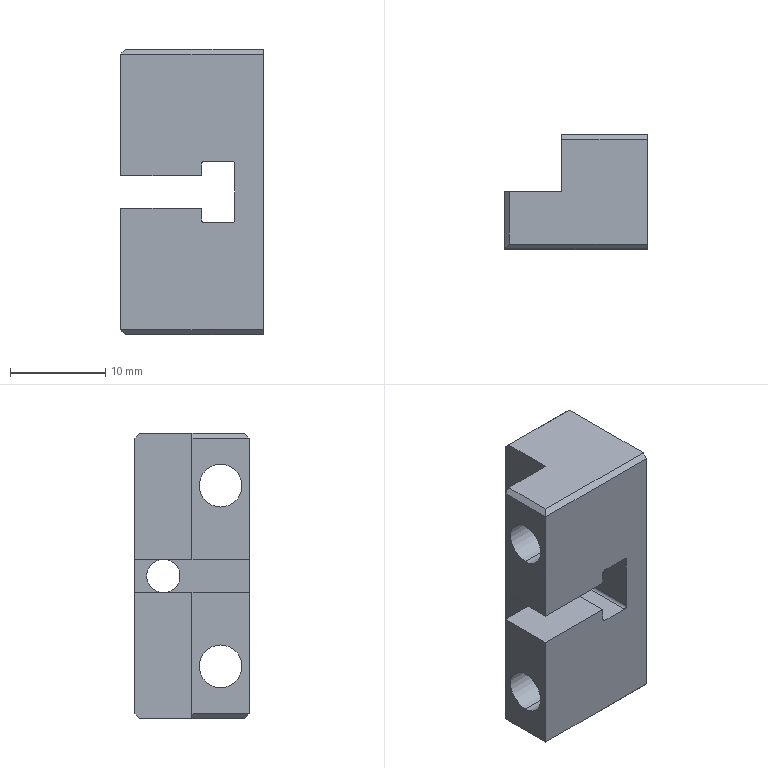Part | NX | features BREP 1 | 1 solid | 34 faces | box 15 x 12 x 30 mm | volume 3310 mm3 | plane 24 | cylinder 10 | commonest cylinder face diameters 0.6 x4 4.5 x4 3.5 x2
STEP:
#1=CARTESIAN_POINT('',(-3.,9.,16.75));
#2=VERTEX_POINT('',#1);
#3=CARTESIAN_POINT('',(-3.,9.,13.25));
#4=VERTEX_POINT('',#3);
#5=CARTESIAN_POINT('',(-3.,9.,15.));
#6=DIRECTION('',(1.,0.,0.));
#7=DIRECTION('',(0.,1.,0.));
#8=AXIS2_PLACEMENT_3D('',#5,#6,#7);
#9=CIRCLE('',#8,1.75);
#10=EDGE_CURVE('',#2,#4,#9,.T.);
#11=ORIENTED_EDGE('',*,*,#10,.F.);
#12=CARTESIAN_POINT('',(0.,9.,16.75));
#13=VERTEX_POINT('',#12);
#14=CARTESIAN_POINT('',(0.,9.,16.75));
#15=DIRECTION('',(1.,0.,0.));
#16=VECTOR('',#15,1000.);
#17=LINE('',#14,#16);
#18=EDGE_CURVE('',#2,#13,#17,.T.);
#19=ORIENTED_EDGE('',*,*,#18,.T.);
#20=CARTESIAN_POINT('',(0.,9.,13.25));
#21=VERTEX_POINT('',#20);
#22=CARTESIAN_POINT('',(0.,9.,15.));
#23=DIRECTION('',(1.,0.,0.));
#24=DIRECTION('',(0.,0.,-1.));
#25=AXIS2_PLACEMENT_3D('',#22,#23,#24);
#26=CIRCLE('',#25,1.75);
#27=EDGE_CURVE('',#13,#21,#26,.T.);
#28=ORIENTED_EDGE('',*,*,#27,.T.);
#29=CARTESIAN_POINT('',(0.,9.,13.25));
#30=DIRECTION('',(1.,0.,0.));
#31=VECTOR('',#30,1000.);
#32=LINE('',#29,#31);
#33=EDGE_CURVE('',#4,#21,#32,.T.);
#34=ORIENTED_EDGE('',*,*,#33,.F.);
#35=EDGE_LOOP('',(#11,#19,#28,#34));
#36=FACE_BOUND('',#35,.T.);
#37=CARTESIAN_POINT('',(0.,9.,15.));
#38=DIRECTION('',(1.,0.,0.));
#39=DIRECTION('',(0.,0.,-1.));
#40=AXIS2_PLACEMENT_3D('',#37,#38,#39);
#41=CYLINDRICAL_SURFACE('',#40,1.75);
#42=ADVANCED_FACE('',(#36),#41,.F.);
#43=CARTESIAN_POINT('',(-15.,3.,26.75));
#44=VERTEX_POINT('',#43);
#45=CARTESIAN_POINT('',(-15.,3.,22.25));
#46=VERTEX_POINT('',#45);
#47=CARTESIAN_POINT('',(-15.,3.,24.5));
#48=DIRECTION('',(1.,0.,0.));
#49=DIRECTION('',(0.,0.,-1.));
#50=AXIS2_PLACEMENT_3D('',#47,#48,#49);
#51=CIRCLE('',#50,2.25);
#52=EDGE_CURVE('',#44,#46,#51,.T.);
#53=ORIENTED_EDGE('',*,*,#52,.F.);
#54=CARTESIAN_POINT('',(0.,3.,26.75));
#55=VERTEX_POINT('',#54);
#56=CARTESIAN_POINT('',(0.,3.,26.75));
#57=DIRECTION('',(1.,0.,0.));
#58=VECTOR('',#57,1000.);
#59=LINE('',#56,#58);
#60=EDGE_CURVE('',#44,#55,#59,.T.);
#61=ORIENTED_EDGE('',*,*,#60,.T.);
#62=CARTESIAN_POINT('',(0.,3.,22.25));
#63=VERTEX_POINT('',#62);
#64=CARTESIAN_POINT('',(0.,3.,24.5));
#65=DIRECTION('',(1.,0.,0.));
#66=DIRECTION('',(0.,0.,-1.));
#67=AXIS2_PLACEMENT_3D('',#64,#65,#66);
#68=CIRCLE('',#67,2.25);
#69=EDGE_CURVE('',#55,#63,#68,.T.);
#70=ORIENTED_EDGE('',*,*,#69,.T.);
#71=CARTESIAN_POINT('',(0.,3.,22.25));
#72=DIRECTION('',(1.,0.,0.));
#73=VECTOR('',#72,1000.);
#74=LINE('',#71,#73);
#75=EDGE_CURVE('',#46,#63,#74,.T.);
#76=ORIENTED_EDGE('',*,*,#75,.F.);
#77=EDGE_LOOP('',(#53,#61,#70,#76));
#78=FACE_BOUND('',#77,.T.);
#79=CARTESIAN_POINT('',(0.,3.,24.5));
#80=DIRECTION('',(1.,0.,0.));
#81=DIRECTION('',(0.,0.,-1.));
#82=AXIS2_PLACEMENT_3D('',#79,#80,#81);
#83=CYLINDRICAL_SURFACE('',#82,2.25);
#84=ADVANCED_FACE('',(#78),#83,.F.);
#85=CARTESIAN_POINT('',(-15.,3.,7.75));
#86=VERTEX_POINT('',#85);
#87=CARTESIAN_POINT('',(-15.,3.,3.25));
#88=VERTEX_POINT('',#87);
#89=CARTESIAN_POINT('',(-15.,3.,5.5));
#90=DIRECTION('',(1.,0.,0.));
#91=DIRECTION('',(0.,0.,-1.));
#92=AXIS2_PLACEMENT_3D('',#89,#90,#91);
#93=CIRCLE('',#92,2.25);
#94=EDGE_CURVE('',#86,#88,#93,.T.);
#95=ORIENTED_EDGE('',*,*,#94,.F.);
#96=CARTESIAN_POINT('',(0.,3.,7.75));
#97=VERTEX_POINT('',#96);
#98=CARTESIAN_POINT('',(0.,3.,7.75));
#99=DIRECTION('',(1.,0.,0.));
#100=VECTOR('',#99,1000.);
#101=LINE('',#98,#100);
#102=EDGE_CURVE('',#86,#97,#101,.T.);
#103=ORIENTED_EDGE('',*,*,#102,.T.);
#104=CARTESIAN_POINT('',(0.,3.,3.25));
#105=VERTEX_POINT('',#104);
#106=CARTESIAN_POINT('',(0.,3.,5.5));
#107=DIRECTION('',(1.,0.,0.));
#108=DIRECTION('',(0.,0.,-1.));
#109=AXIS2_PLACEMENT_3D('',#106,#107,#108);
#110=CIRCLE('',#109,2.25);
#111=EDGE_CURVE('',#97,#105,#110,.T.);
#112=ORIENTED_EDGE('',*,*,#111,.T.);
#113=CARTESIAN_POINT('',(0.,3.,3.25));
#114=DIRECTION('',(1.,0.,0.));
#115=VECTOR('',#114,1000.);
#116=LINE('',#113,#115);
#117=EDGE_CURVE('',#88,#105,#116,.T.);
#118=ORIENTED_EDGE('',*,*,#117,.F.);
#119=EDGE_LOOP('',(#95,#103,#112,#118));
#120=FACE_BOUND('',#119,.T.);
#121=CARTESIAN_POINT('',(0.,3.,5.5));
#122=DIRECTION('',(1.,0.,0.));
#123=DIRECTION('',(0.,0.,-1.));
#124=AXIS2_PLACEMENT_3D('',#121,#122,#123);
#125=CYLINDRICAL_SURFACE('',#124,2.25);
#126=ADVANCED_FACE('',(#120),#125,.F.);
#127=CARTESIAN_POINT('',(-9.,6.,30.));
#128=VERTEX_POINT('',#127);
#129=CARTESIAN_POINT('',(-9.,6.,16.7));
#130=VERTEX_POINT('',#129);
#131=CARTESIAN_POINT('',(-9.,6.,30.));
#132=DIRECTION('',(0.,0.,-1.));
#133=VECTOR('',#132,1000.);
#134=LINE('',#131,#133);
#135=EDGE_CURVE('',#128,#130,#134,.T.);
#136=ORIENTED_EDGE('',*,*,#135,.T.);
#137=CARTESIAN_POINT('',(-15.,6.,16.7));
#138=VERTEX_POINT('',#137);
#139=CARTESIAN_POINT('',(-9.,6.,16.7));
#140=DIRECTION('',(1.,0.,0.));
#141=VECTOR('',#140,1000.);
#142=LINE('',#139,#141);
#143=EDGE_CURVE('',#138,#130,#142,.T.);
#144=ORIENTED_EDGE('',*,*,#143,.F.);
#145=CARTESIAN_POINT('',(-15.,6.,29.5));
#146=VERTEX_POINT('',#145);
#147=CARTESIAN_POINT('',(-15.,6.,30.));
#148=DIRECTION('',(0.,0.,-1.));
#149=VECTOR('',#148,1000.);
#150=LINE('',#147,#149);
#151=EDGE_CURVE('',#146,#138,#150,.T.);
#152=ORIENTED_EDGE('',*,*,#151,.F.);
#153=CARTESIAN_POINT('',(-14.5,6.,30.));
#154=VERTEX_POINT('',#153);
#155=CARTESIAN_POINT('',(-14.5,6.,30.));
#156=DIRECTION('',(0.7071,0.,0.7071));
#157=VECTOR('',#156,1000.);
#158=LINE('',#155,#157);
#159=EDGE_CURVE('',#146,#154,#158,.T.);
#160=ORIENTED_EDGE('',*,*,#159,.T.);
#161=CARTESIAN_POINT('',(-9.,6.,30.));
#162=DIRECTION('',(-1.,0.,0.));
#163=VECTOR('',#162,1000.);
#164=LINE('',#161,#163);
#165=EDGE_CURVE('',#128,#154,#164,.T.);
#166=ORIENTED_EDGE('',*,*,#165,.F.);
#167=EDGE_LOOP('',(#136,#144,#152,#160,#166));
#168=FACE_BOUND('',#167,.T.);
#169=CARTESIAN_POINT('',(-9.,6.,30.));
#170=DIRECTION('',(0.,-1.,0.));
#171=DIRECTION('',(0.,0.,-1.));
#172=AXIS2_PLACEMENT_3D('',#169,#170,#171);
#173=PLANE('',#172);
#174=ADVANCED_FACE('',(#168),#173,.F.);
#175=ORIENTED_EDGE('',*,*,#151,.T.);
#176=CARTESIAN_POINT('',(-15.,0.,16.7));
#177=VERTEX_POINT('',#176);
#178=CARTESIAN_POINT('',(-15.,0.,16.7));
#179=DIRECTION('',(0.,1.,0.));
#180=VECTOR('',#179,1000.);
#181=LINE('',#178,#180);
#182=EDGE_CURVE('',#177,#138,#181,.T.);
#183=ORIENTED_EDGE('',*,*,#182,.F.);
#184=CARTESIAN_POINT('',(-15.,0.,29.5));
#185=VERTEX_POINT('',#184);
#186=CARTESIAN_POINT('',(-15.,0.,30.));
#187=DIRECTION('',(0.,0.,-1.));
#188=VECTOR('',#187,1000.);
#189=LINE('',#186,#188);
#190=EDGE_CURVE('',#185,#177,#189,.T.);
#191=ORIENTED_EDGE('',*,*,#190,.F.);
#192=CARTESIAN_POINT('',(-15.,6.,29.5));
#193=DIRECTION('',(0.,1.,0.));
#194=VECTOR('',#193,1000.);
#195=LINE('',#192,#194);
#196=EDGE_CURVE('',#185,#146,#195,.T.);
#197=ORIENTED_EDGE('',*,*,#196,.T.);
#198=EDGE_LOOP('',(#175,#183,#191,#197));
#199=FACE_BOUND('',#198,.T.);
#200=CARTESIAN_POINT('',(-15.,3.,24.5));
#201=DIRECTION('',(1.,0.,0.));
#202=DIRECTION('',(0.,0.,-1.));
#203=AXIS2_PLACEMENT_3D('',#200,#201,#202);
#204=CIRCLE('',#203,2.25);
#205=EDGE_CURVE('',#46,#44,#204,.T.);
#206=ORIENTED_EDGE('',*,*,#205,.T.);
#207=ORIENTED_EDGE('',*,*,#52,.T.);
#208=EDGE_LOOP('',(#206,#207));
#209=FACE_BOUND('',#208,.T.);
#210=CARTESIAN_POINT('',(-15.,6.,30.));
#211=DIRECTION('',(1.,0.,0.));
#212=DIRECTION('',(0.,1.,0.));
#213=AXIS2_PLACEMENT_3D('',#210,#211,#212);
#214=PLANE('',#213);
#215=ADVANCED_FACE('',(#199,#209),#214,.F.);
#216=CARTESIAN_POINT('',(0.,0.,29.5));
#217=VERTEX_POINT('',#216);
#218=CARTESIAN_POINT('',(0.,0.,0.5));
#219=VERTEX_POINT('',#218);
#220=CARTESIAN_POINT('',(0.,0.,30.));
#221=DIRECTION('',(0.,0.,-1.));
#222=VECTOR('',#221,1000.);
#223=LINE('',#220,#222);
#224=EDGE_CURVE('',#217,#219,#223,.T.);
#225=ORIENTED_EDGE('',*,*,#224,.T.);
#226=CARTESIAN_POINT('',(0.,0.5,0.));
#227=VERTEX_POINT('',#226);
#228=CARTESIAN_POINT('',(0.,0.,0.5));
#229=DIRECTION('',(0.,0.7071,-0.7071));
#230=VECTOR('',#229,1000.);
#231=LINE('',#228,#230);
#232=EDGE_CURVE('',#219,#227,#231,.T.);
#233=ORIENTED_EDGE('',*,*,#232,.T.);
#234=CARTESIAN_POINT('',(0.,11.5,0.));
#235=VERTEX_POINT('',#234);
#236=CARTESIAN_POINT('',(0.,0.,0.));
#237=DIRECTION('',(0.,1.,0.));
#238=VECTOR('',#237,1000.);
#239=LINE('',#236,#238);
#240=EDGE_CURVE('',#227,#235,#239,.T.);
#241=ORIENTED_EDGE('',*,*,#240,.T.);
#242=CARTESIAN_POINT('',(0.,12.,0.5));
#243=VERTEX_POINT('',#242);
#244=CARTESIAN_POINT('',(0.,12.,0.5));
#245=DIRECTION('',(0.,0.7071,0.7071));
#246=VECTOR('',#245,1000.);
#247=LINE('',#244,#246);
#248=EDGE_CURVE('',#235,#243,#247,.T.);
#249=ORIENTED_EDGE('',*,*,#248,.T.);
#250=CARTESIAN_POINT('',(0.,12.,29.5));
#251=VERTEX_POINT('',#250);
#252=CARTESIAN_POINT('',(0.,12.,30.));
#253=DIRECTION('',(0.,0.,-1.));
#254=VECTOR('',#253,1000.);
#255=LINE('',#252,#254);
#256=EDGE_CURVE('',#251,#243,#255,.T.);
#257=ORIENTED_EDGE('',*,*,#256,.F.);
#258=CARTESIAN_POINT('',(0.,11.5,30.));
#259=VERTEX_POINT('',#258);
#260=CARTESIAN_POINT('',(0.,11.5,30.));
#261=DIRECTION('',(0.,-0.7071,0.7071));
#262=VECTOR('',#261,1000.);
#263=LINE('',#260,#262);
#264=EDGE_CURVE('',#251,#259,#263,.T.);
#265=ORIENTED_EDGE('',*,*,#264,.T.);
#266=CARTESIAN_POINT('',(0.,0.5,30.));
#267=VERTEX_POINT('',#266);
#268=CARTESIAN_POINT('',(0.,0.,30.));
#269=DIRECTION('',(0.,1.,0.));
#270=VECTOR('',#269,1000.);
#271=LINE('',#268,#270);
#272=EDGE_CURVE('',#267,#259,#271,.T.);
#273=ORIENTED_EDGE('',*,*,#272,.F.);
#274=CARTESIAN_POINT('',(0.,0.5,30.));
#275=DIRECTION('',(0.,-0.7071,-0.7071));
#276=VECTOR('',#275,1000.);
#277=LINE('',#274,#276);
#278=EDGE_CURVE('',#267,#217,#277,.T.);
#279=ORIENTED_EDGE('',*,*,#278,.T.);
#280=EDGE_LOOP('',(#225,#233,#241,#249,#257,#265,#273,#279));
#281=FACE_BOUND('',#280,.T.);
#282=CARTESIAN_POINT('',(0.,3.,5.5));
#283=DIRECTION('',(1.,0.,0.));
#284=DIRECTION('',(0.,0.,-1.));
#285=AXIS2_PLACEMENT_3D('',#282,#283,#284);
#286=CIRCLE('',#285,2.25);
#287=EDGE_CURVE('',#105,#97,#286,.T.);
#288=ORIENTED_EDGE('',*,*,#287,.F.);
#289=ORIENTED_EDGE('',*,*,#111,.F.);
#290=EDGE_LOOP('',(#288,#289));
#291=FACE_BOUND('',#290,.T.);
#292=CARTESIAN_POINT('',(0.,3.,24.5));
#293=DIRECTION('',(1.,0.,0.));
#294=DIRECTION('',(0.,0.,-1.));
#295=AXIS2_PLACEMENT_3D('',#292,#293,#294);
#296=CIRCLE('',#295,2.25);
#297=EDGE_CURVE('',#63,#55,#296,.T.);
#298=ORIENTED_EDGE('',*,*,#297,.F.);
#299=ORIENTED_EDGE('',*,*,#69,.F.);
#300=EDGE_LOOP('',(#298,#299));
#301=FACE_BOUND('',#300,.T.);
#302=CARTESIAN_POINT('',(0.,9.,15.));
#303=DIRECTION('',(1.,0.,0.));
#304=DIRECTION('',(0.,0.,-1.));
#305=AXIS2_PLACEMENT_3D('',#302,#303,#304);
#306=CIRCLE('',#305,1.75);
#307=EDGE_CURVE('',#21,#13,#306,.T.);
#308=ORIENTED_EDGE('',*,*,#307,.F.);
#309=ORIENTED_EDGE('',*,*,#27,.F.);
#310=EDGE_LOOP('',(#308,#309));
#311=FACE_BOUND('',#310,.T.);
#312=CARTESIAN_POINT('',(0.,0.,30.));
#313=DIRECTION('',(-1.,0.,0.));
#314=DIRECTION('',(0.,0.,1.));
#315=AXIS2_PLACEMENT_3D('',#312,#313,#314);
#316=PLANE('',#315);
#317=ADVANCED_FACE('',(#281,#291,#301,#311),#316,.F.);
#318=CARTESIAN_POINT('',(-9.,6.,13.3));
#319=VERTEX_POINT('',#318);
#320=CARTESIAN_POINT('',(-9.,6.,0.));
#321=VERTEX_POINT('',#320);
#322=CARTESIAN_POINT('',(-9.,6.,30.));
#323=DIRECTION('',(0.,0.,-1.));
#324=VECTOR('',#323,1000.);
#325=LINE('',#322,#324);
#326=EDGE_CURVE('',#319,#321,#325,.T.);
#327=ORIENTED_EDGE('',*,*,#326,.F.);
#328=CARTESIAN_POINT('',(-9.,12.,13.3));
#329=VERTEX_POINT('',#328);
#330=CARTESIAN_POINT('',(-9.,0.,13.3));
#331=DIRECTION('',(0.,1.,0.));
#332=VECTOR('',#331,1000.);
#333=LINE('',#330,#332);
#334=EDGE_CURVE('',#319,#329,#333,.T.);
#335=ORIENTED_EDGE('',*,*,#334,.T.);
#336=CARTESIAN_POINT('',(-9.,12.,0.5));
#337=VERTEX_POINT('',#336);
#338=CARTESIAN_POINT('',(-9.,12.,30.));
#339=DIRECTION('',(0.,0.,-1.));
#340=VECTOR('',#339,1000.);
#341=LINE('',#338,#340);
#342=EDGE_CURVE('',#329,#337,#341,.T.);
#343=ORIENTED_EDGE('',*,*,#342,.T.);
#344=CARTESIAN_POINT('',(-9.,11.5,0.));
#345=VERTEX_POINT('',#344);
#346=CARTESIAN_POINT('',(-9.,12.,0.5));
#347=DIRECTION('',(0.,-0.7071,-0.7071));
#348=VECTOR('',#347,1000.);
#349=LINE('',#346,#348);
#350=EDGE_CURVE('',#337,#345,#349,.T.);
#351=ORIENTED_EDGE('',*,*,#350,.T.);
#352=CARTESIAN_POINT('',(-9.,12.,0.));
#353=DIRECTION('',(0.,-1.,0.));
#354=VECTOR('',#353,1000.);
#355=LINE('',#352,#354);
#356=EDGE_CURVE('',#345,#321,#355,.T.);
#357=ORIENTED_EDGE('',*,*,#356,.T.);
#358=EDGE_LOOP('',(#327,#335,#343,#351,#357));
#359=FACE_BOUND('',#358,.T.);
#360=CARTESIAN_POINT('',(-9.,12.,30.));
#361=DIRECTION('',(1.,0.,0.));
#362=DIRECTION('',(0.,1.,0.));
#363=AXIS2_PLACEMENT_3D('',#360,#361,#362);
#364=PLANE('',#363);
#365=ADVANCED_FACE('',(#359),#364,.F.);
#366=ORIENTED_EDGE('',*,*,#342,.F.);
#367=CARTESIAN_POINT('',(-6.5,12.,13.3));
#368=VERTEX_POINT('',#367);
#369=CARTESIAN_POINT('',(-9.,12.,13.3));
#370=DIRECTION('',(-1.,0.,0.));
#371=VECTOR('',#370,1000.);
#372=LINE('',#369,#371);
#373=EDGE_CURVE('',#368,#329,#372,.T.);
#374=ORIENTED_EDGE('',*,*,#373,.F.);
#375=CARTESIAN_POINT('',(-6.5,12.,12.05));
#376=VERTEX_POINT('',#375);
#377=CARTESIAN_POINT('',(-6.5,12.,13.3));
#378=DIRECTION('',(0.,0.,1.));
#379=VECTOR('',#378,1000.);
#380=LINE('',#377,#379);
#381=EDGE_CURVE('',#376,#368,#380,.T.);
#382=ORIENTED_EDGE('',*,*,#381,.F.);
#383=CARTESIAN_POINT('',(-6.2,12.,11.75));
#384=VERTEX_POINT('',#383);
#385=CARTESIAN_POINT('',(-6.2,12.,12.05));
#386=DIRECTION('',(0.,-1.,0.));
#387=DIRECTION('',(1.,0.,0.));
#388=AXIS2_PLACEMENT_3D('',#385,#386,#387);
#389=CIRCLE('',#388,0.3);
#390=EDGE_CURVE('',#376,#384,#389,.T.);
#391=ORIENTED_EDGE('',*,*,#390,.T.);
#392=CARTESIAN_POINT('',(-3.3,12.,11.75));
#393=VERTEX_POINT('',#392);
#394=CARTESIAN_POINT('',(-6.5,12.,11.75));
#395=DIRECTION('',(-1.,0.,0.));
#396=VECTOR('',#395,1000.);
#397=LINE('',#394,#396);
#398=EDGE_CURVE('',#393,#384,#397,.T.);
#399=ORIENTED_EDGE('',*,*,#398,.F.);
#400=CARTESIAN_POINT('',(-3.,12.,12.05));
#401=VERTEX_POINT('',#400);
#402=CARTESIAN_POINT('',(-3.3,12.,12.05));
#403=DIRECTION('',(0.,-1.,0.));
#404=DIRECTION('',(1.,0.,0.));
#405=AXIS2_PLACEMENT_3D('',#402,#403,#404);
#406=CIRCLE('',#405,0.3);
#407=EDGE_CURVE('',#393,#401,#406,.T.);
#408=ORIENTED_EDGE('',*,*,#407,.T.);
#409=CARTESIAN_POINT('',(-3.,12.,17.95));
#410=VERTEX_POINT('',#409);
#411=CARTESIAN_POINT('',(-3.,12.,11.75));
#412=DIRECTION('',(0.,0.,-1.));
#413=VECTOR('',#412,1000.);
#414=LINE('',#411,#413);
#415=EDGE_CURVE('',#410,#401,#414,.T.);
#416=ORIENTED_EDGE('',*,*,#415,.F.);
#417=CARTESIAN_POINT('',(-3.3,12.,18.25));
#418=VERTEX_POINT('',#417);
#419=CARTESIAN_POINT('',(-3.3,12.,17.95));
#420=DIRECTION('',(0.,-1.,0.));
#421=DIRECTION('',(1.,0.,0.));
#422=AXIS2_PLACEMENT_3D('',#419,#420,#421);
#423=CIRCLE('',#422,0.3);
#424=EDGE_CURVE('',#410,#418,#423,.T.);
#425=ORIENTED_EDGE('',*,*,#424,.T.);
#426=CARTESIAN_POINT('',(-6.2,12.,18.25));
#427=VERTEX_POINT('',#426);
#428=CARTESIAN_POINT('',(-3.,12.,18.25));
#429=DIRECTION('',(1.,0.,0.));
#430=VECTOR('',#429,1000.);
#431=LINE('',#428,#430);
#432=EDGE_CURVE('',#427,#418,#431,.T.);
#433=ORIENTED_EDGE('',*,*,#432,.F.);
#434=CARTESIAN_POINT('',(-6.5,12.,17.95));
#435=VERTEX_POINT('',#434);
#436=CARTESIAN_POINT('',(-6.2,12.,17.95));
#437=DIRECTION('',(0.,-1.,0.));
#438=DIRECTION('',(1.,0.,0.));
#439=AXIS2_PLACEMENT_3D('',#436,#437,#438);
#440=CIRCLE('',#439,0.3);
#441=EDGE_CURVE('',#427,#435,#440,.T.);
#442=ORIENTED_EDGE('',*,*,#441,.T.);
#443=CARTESIAN_POINT('',(-6.5,12.,16.7));
#444=VERTEX_POINT('',#443);
#445=CARTESIAN_POINT('',(-6.5,12.,18.25));
#446=DIRECTION('',(0.,0.,1.));
#447=VECTOR('',#446,1000.);
#448=LINE('',#445,#447);
#449=EDGE_CURVE('',#444,#435,#448,.T.);
#450=ORIENTED_EDGE('',*,*,#449,.F.);
#451=CARTESIAN_POINT('',(-9.,12.,16.7));
#452=VERTEX_POINT('',#451);
#453=CARTESIAN_POINT('',(-6.5,12.,16.7));
#454=DIRECTION('',(1.,0.,0.));
#455=VECTOR('',#454,1000.);
#456=LINE('',#453,#455);
#457=EDGE_CURVE('',#452,#444,#456,.T.);
#458=ORIENTED_EDGE('',*,*,#457,.F.);
#459=CARTESIAN_POINT('',(-9.,12.,29.5));
#460=VERTEX_POINT('',#459);
#461=CARTESIAN_POINT('',(-9.,12.,30.));
#462=DIRECTION('',(0.,0.,-1.));
#463=VECTOR('',#462,1000.);
#464=LINE('',#461,#463);
#465=EDGE_CURVE('',#460,#452,#464,.T.);
#466=ORIENTED_EDGE('',*,*,#465,.F.);
#467=CARTESIAN_POINT('',(0.,12.,29.5));
#468=DIRECTION('',(1.,0.,0.));
#469=VECTOR('',#468,1000.);
#470=LINE('',#467,#469);
#471=EDGE_CURVE('',#460,#251,#470,.T.);
#472=ORIENTED_EDGE('',*,*,#471,.T.);
#473=ORIENTED_EDGE('',*,*,#256,.T.);
#474=CARTESIAN_POINT('',(0.,12.,0.5));
#475=DIRECTION('',(-1.,0.,0.));
#476=VECTOR('',#475,1000.);
#477=LINE('',#474,#476);
#478=EDGE_CURVE('',#243,#337,#477,.T.);
#479=ORIENTED_EDGE('',*,*,#478,.T.);
#480=EDGE_LOOP('',(#366,#374,#382,#391,#399,#408,#416,#425,#433,#442,#450,#458,#466,#472,#473,#479));
#481=FACE_BOUND('',#480,.T.);
#482=CARTESIAN_POINT('',(0.,12.,30.));
#483=DIRECTION('',(0.,-1.,0.));
#484=DIRECTION('',(0.,0.,-1.));
#485=AXIS2_PLACEMENT_3D('',#482,#483,#484);
#486=PLANE('',#485);
#487=ADVANCED_FACE('',(#481),#486,.F.);
#488=ORIENTED_EDGE('',*,*,#465,.T.);
#489=CARTESIAN_POINT('',(-9.,0.,16.7));
#490=DIRECTION('',(0.,1.,0.));
#491=VECTOR('',#490,1000.);
#492=LINE('',#489,#491);
#493=EDGE_CURVE('',#130,#452,#492,.T.);
#494=ORIENTED_EDGE('',*,*,#493,.F.);
#495=ORIENTED_EDGE('',*,*,#135,.F.);
#496=CARTESIAN_POINT('',(-9.,11.5,30.));
#497=VERTEX_POINT('',#496);
#498=CARTESIAN_POINT('',(-9.,12.,30.));
#499=DIRECTION('',(0.,-1.,0.));
#500=VECTOR('',#499,1000.);
#501=LINE('',#498,#500);
#502=EDGE_CURVE('',#497,#128,#501,.T.);
#503=ORIENTED_EDGE('',*,*,#502,.F.);
#504=CARTESIAN_POINT('',(-9.,11.5,30.));
#505=DIRECTION('',(0.,0.7071,-0.7071));
#506=VECTOR('',#505,1000.);
#507=LINE('',#504,#506);
#508=EDGE_CURVE('',#497,#460,#507,.T.);
#509=ORIENTED_EDGE('',*,*,#508,.T.);
#510=EDGE_LOOP('',(#488,#494,#495,#503,#509));
#511=FACE_BOUND('',#510,.T.);
#512=CARTESIAN_POINT('',(-9.,12.,30.));
#513=DIRECTION('',(1.,0.,0.));
#514=DIRECTION('',(0.,1.,0.));
#515=AXIS2_PLACEMENT_3D('',#512,#513,#514);
#516=PLANE('',#515);
#517=ADVANCED_FACE('',(#511),#516,.F.);
#518=CARTESIAN_POINT('',(-15.,6.,13.3));
#519=VERTEX_POINT('',#518);
#520=CARTESIAN_POINT('',(-15.,6.,0.5));
#521=VERTEX_POINT('',#520);
#522=CARTESIAN_POINT('',(-15.,6.,30.));
#523=DIRECTION('',(0.,0.,-1.));
#524=VECTOR('',#523,1000.);
#525=LINE('',#522,#524);
#526=EDGE_CURVE('',#519,#521,#525,.T.);
#527=ORIENTED_EDGE('',*,*,#526,.F.);
#528=CARTESIAN_POINT('',(-9.,6.,13.3));
#529=DIRECTION('',(-1.,0.,0.));
#530=VECTOR('',#529,1000.);
#531=LINE('',#528,#530);
#532=EDGE_CURVE('',#319,#519,#531,.T.);
#533=ORIENTED_EDGE('',*,*,#532,.F.);
#534=ORIENTED_EDGE('',*,*,#326,.T.);
#535=CARTESIAN_POINT('',(-14.5,6.,0.));
#536=VERTEX_POINT('',#535);
#537=CARTESIAN_POINT('',(-9.,6.,0.));
#538=DIRECTION('',(-1.,0.,0.));
#539=VECTOR('',#538,1000.);
#540=LINE('',#537,#539);
#541=EDGE_CURVE('',#321,#536,#540,.T.);
#542=ORIENTED_EDGE('',*,*,#541,.T.);
#543=CARTESIAN_POINT('',(-15.,6.,0.5));
#544=DIRECTION('',(-0.7071,0.,0.7071));
#545=VECTOR('',#544,1000.);
#546=LINE('',#543,#545);
#547=EDGE_CURVE('',#536,#521,#546,.T.);
#548=ORIENTED_EDGE('',*,*,#547,.T.);
#549=EDGE_LOOP('',(#527,#533,#534,#542,#548));
#550=FACE_BOUND('',#549,.T.);
#551=CARTESIAN_POINT('',(-9.,6.,30.));
#552=DIRECTION('',(0.,-1.,0.));
#553=DIRECTION('',(0.,0.,-1.));
#554=AXIS2_PLACEMENT_3D('',#551,#552,#553);
#555=PLANE('',#554);
#556=ADVANCED_FACE('',(#550),#555,.F.);
#557=CARTESIAN_POINT('',(-15.,0.,13.3));
#558=VERTEX_POINT('',#557);
#559=CARTESIAN_POINT('',(-15.,0.,0.5));
#560=VERTEX_POINT('',#559);
#561=CARTESIAN_POINT('',(-15.,0.,30.));
#562=DIRECTION('',(0.,0.,-1.));
#563=VECTOR('',#562,1000.);
#564=LINE('',#561,#563);
#565=EDGE_CURVE('',#558,#560,#564,.T.);
#566=ORIENTED_EDGE('',*,*,#565,.F.);
#567=CARTESIAN_POINT('',(-15.,0.,13.3));
#568=DIRECTION('',(0.,1.,0.));
#569=VECTOR('',#568,1000.);
#570=LINE('',#567,#569);
#571=EDGE_CURVE('',#558,#519,#570,.T.);
#572=ORIENTED_EDGE('',*,*,#571,.T.);
#573=ORIENTED_EDGE('',*,*,#526,.T.);
#574=CARTESIAN_POINT('',(-15.,6.,0.5));
#575=DIRECTION('',(0.,-1.,0.));
#576=VECTOR('',#575,1000.);
#577=LINE('',#574,#576);
#578=EDGE_CURVE('',#521,#560,#577,.T.);
#579=ORIENTED_EDGE('',*,*,#578,.T.);
#580=EDGE_LOOP('',(#566,#572,#573,#579));
#581=FACE_BOUND('',#580,.T.);
#582=CARTESIAN_POINT('',(-15.,3.,5.5));
#583=DIRECTION('',(1.,0.,0.));
#584=DIRECTION('',(0.,0.,-1.));
#585=AXIS2_PLACEMENT_3D('',#582,#583,#584);
#586=CIRCLE('',#585,2.25);
#587=EDGE_CURVE('',#88,#86,#586,.T.);
#588=ORIENTED_EDGE('',*,*,#587,.T.);
#589=ORIENTED_EDGE('',*,*,#94,.T.);
#590=EDGE_LOOP('',(#588,#589));
#591=FACE_BOUND('',#590,.T.);
#592=CARTESIAN_POINT('',(-15.,6.,30.));
#593=DIRECTION('',(1.,0.,0.));
#594=DIRECTION('',(0.,1.,0.));
#595=AXIS2_PLACEMENT_3D('',#592,#593,#594);
#596=PLANE('',#595);
#597=ADVANCED_FACE('',(#581,#591),#596,.F.);
#598=ORIENTED_EDGE('',*,*,#190,.T.);
#599=CARTESIAN_POINT('',(-6.5,0.,16.7));
#600=VERTEX_POINT('',#599);
#601=CARTESIAN_POINT('',(-6.5,0.,16.7));
#602=DIRECTION('',(1.,0.,0.));
#603=VECTOR('',#602,1000.);
#604=LINE('',#601,#603);
#605=EDGE_CURVE('',#177,#600,#604,.T.);
#606=ORIENTED_EDGE('',*,*,#605,.T.);
#607=CARTESIAN_POINT('',(-6.5,0.,17.95));
#608=VERTEX_POINT('',#607);
#609=CARTESIAN_POINT('',(-6.5,0.,18.25));
#610=DIRECTION('',(0.,0.,1.));
#611=VECTOR('',#610,1000.);
#612=LINE('',#609,#611);
#613=EDGE_CURVE('',#600,#608,#612,.T.);
#614=ORIENTED_EDGE('',*,*,#613,.T.);
#615=CARTESIAN_POINT('',(-6.2,0.,18.25));
#616=VERTEX_POINT('',#615);
#617=CARTESIAN_POINT('',(-6.2,0.,17.95));
#618=DIRECTION('',(0.,1.,0.));
#619=DIRECTION('',(-1.,0.,0.));
#620=AXIS2_PLACEMENT_3D('',#617,#618,#619);
#621=CIRCLE('',#620,0.3);
#622=EDGE_CURVE('',#608,#616,#621,.T.);
#623=ORIENTED_EDGE('',*,*,#622,.T.);
#624=CARTESIAN_POINT('',(-3.3,0.,18.25));
#625=VERTEX_POINT('',#624);
#626=CARTESIAN_POINT('',(-3.,0.,18.25));
#627=DIRECTION('',(1.,0.,0.));
#628=VECTOR('',#627,1000.);
#629=LINE('',#626,#628);
#630=EDGE_CURVE('',#616,#625,#629,.T.);
#631=ORIENTED_EDGE('',*,*,#630,.T.);
#632=CARTESIAN_POINT('',(-3.,0.,17.95));
#633=VERTEX_POINT('',#632);
#634=CARTESIAN_POINT('',(-3.3,0.,17.95));
#635=DIRECTION('',(0.,1.,0.));
#636=DIRECTION('',(-1.,0.,0.));
#637=AXIS2_PLACEMENT_3D('',#634,#635,#636);
#638=CIRCLE('',#637,0.3);
#639=EDGE_CURVE('',#625,#633,#638,.T.);
#640=ORIENTED_EDGE('',*,*,#639,.T.);
#641=CARTESIAN_POINT('',(-3.,0.,12.05));
#642=VERTEX_POINT('',#641);
#643=CARTESIAN_POINT('',(-3.,0.,11.75));
#644=DIRECTION('',(0.,0.,-1.));
#645=VECTOR('',#644,1000.);
#646=LINE('',#643,#645);
#647=EDGE_CURVE('',#633,#642,#646,.T.);
#648=ORIENTED_EDGE('',*,*,#647,.T.);
#649=CARTESIAN_POINT('',(-3.3,0.,11.75));
#650=VERTEX_POINT('',#649);
#651=CARTESIAN_POINT('',(-3.3,0.,12.05));
#652=DIRECTION('',(0.,1.,0.));
#653=DIRECTION('',(-1.,0.,0.));
#654=AXIS2_PLACEMENT_3D('',#651,#652,#653);
#655=CIRCLE('',#654,0.3);
#656=EDGE_CURVE('',#642,#650,#655,.T.);
#657=ORIENTED_EDGE('',*,*,#656,.T.);
#658=CARTESIAN_POINT('',(-6.2,0.,11.75));
#659=VERTEX_POINT('',#658);
#660=CARTESIAN_POINT('',(-6.5,0.,11.75));
#661=DIRECTION('',(-1.,0.,0.));
#662=VECTOR('',#661,1000.);
#663=LINE('',#660,#662);
#664=EDGE_CURVE('',#650,#659,#663,.T.);
#665=ORIENTED_EDGE('',*,*,#664,.T.);
#666=CARTESIAN_POINT('',(-6.5,0.,12.05));
#667=VERTEX_POINT('',#666);
#668=CARTESIAN_POINT('',(-6.2,0.,12.05));
#669=DIRECTION('',(0.,1.,0.));
#670=DIRECTION('',(-1.,0.,0.));
#671=AXIS2_PLACEMENT_3D('',#668,#669,#670);
#672=CIRCLE('',#671,0.3);
#673=EDGE_CURVE('',#659,#667,#672,.T.);
#674=ORIENTED_EDGE('',*,*,#673,.T.);
#675=CARTESIAN_POINT('',(-6.5,0.,13.3));
#676=VERTEX_POINT('',#675);
#677=CARTESIAN_POINT('',(-6.5,0.,13.3));
#678=DIRECTION('',(0.,0.,1.));
#679=VECTOR('',#678,1000.);
#680=LINE('',#677,#679);
#681=EDGE_CURVE('',#667,#676,#680,.T.);
#682=ORIENTED_EDGE('',*,*,#681,.T.);
#683=CARTESIAN_POINT('',(-9.,0.,13.3));
#684=DIRECTION('',(-1.,0.,0.));
#685=VECTOR('',#684,1000.);
#686=LINE('',#683,#685);
#687=EDGE_CURVE('',#676,#558,#686,.T.);
#688=ORIENTED_EDGE('',*,*,#687,.T.);
#689=ORIENTED_EDGE('',*,*,#565,.T.);
#690=CARTESIAN_POINT('',(0.,0.,0.5));
#691=DIRECTION('',(1.,0.,0.));
#692=VECTOR('',#691,1000.);
#693=LINE('',#690,#692);
#694=EDGE_CURVE('',#560,#219,#693,.T.);
#695=ORIENTED_EDGE('',*,*,#694,.T.);
#696=ORIENTED_EDGE('',*,*,#224,.F.);
#697=CARTESIAN_POINT('',(-15.,0.,29.5));
#698=DIRECTION('',(-1.,0.,0.));
#699=VECTOR('',#698,1000.);
#700=LINE('',#697,#699);
#701=EDGE_CURVE('',#217,#185,#700,.T.);
#702=ORIENTED_EDGE('',*,*,#701,.T.);
#703=EDGE_LOOP('',(#598,#606,#614,#623,#631,#640,#648,#657,#665,#674,#682,#688,#689,#695,#696,#702));
#704=FACE_BOUND('',#703,.T.);
#705=CARTESIAN_POINT('',(0.,0.,30.));
#706=DIRECTION('',(0.,1.,0.));
#707=DIRECTION('',(1.,0.,0.));
#708=AXIS2_PLACEMENT_3D('',#705,#706,#707);
#709=PLANE('',#708);
#710=ADVANCED_FACE('',(#704),#709,.F.);
#711=ORIENTED_EDGE('',*,*,#272,.T.);
#712=CARTESIAN_POINT('',(-9.,11.5,30.));
#713=DIRECTION('',(-1.,0.,0.));
#714=VECTOR('',#713,1000.);
#715=LINE('',#712,#714);
#716=EDGE_CURVE('',#259,#497,#715,.T.);
#717=ORIENTED_EDGE('',*,*,#716,.T.);
#718=ORIENTED_EDGE('',*,*,#502,.T.);
#719=ORIENTED_EDGE('',*,*,#165,.T.);
#720=CARTESIAN_POINT('',(-14.5,0.5,30.));
#721=VERTEX_POINT('',#720);
#722=CARTESIAN_POINT('',(-14.5,0.,30.));
#723=DIRECTION('',(0.,-1.,0.));
#724=VECTOR('',#723,1000.);
#725=LINE('',#722,#724);
#726=EDGE_CURVE('',#154,#721,#725,.T.);
#727=ORIENTED_EDGE('',*,*,#726,.T.);
#728=CARTESIAN_POINT('',(0.,0.5,30.));
#729=DIRECTION('',(1.,0.,0.));
#730=VECTOR('',#729,1000.);
#731=LINE('',#728,#730);
#732=EDGE_CURVE('',#721,#267,#731,.T.);
#733=ORIENTED_EDGE('',*,*,#732,.T.);
#734=EDGE_LOOP('',(#711,#717,#718,#719,#727,#733));
#735=FACE_BOUND('',#734,.T.);
#736=CARTESIAN_POINT('',(0.,0.,30.));
#737=DIRECTION('',(0.,0.,1.));
#738=DIRECTION('',(1.,0.,0.));
#739=AXIS2_PLACEMENT_3D('',#736,#737,#738);
#740=PLANE('',#739);
#741=ADVANCED_FACE('',(#735),#740,.T.);
#742=ORIENTED_EDGE('',*,*,#240,.F.);
#743=CARTESIAN_POINT('',(-14.5,0.5,0.));
#744=VERTEX_POINT('',#743);
#745=CARTESIAN_POINT('',(0.,0.5,0.));
#746=DIRECTION('',(-1.,0.,0.));
#747=VECTOR('',#746,1000.);
#748=LINE('',#745,#747);
#749=EDGE_CURVE('',#227,#744,#748,.T.);
#750=ORIENTED_EDGE('',*,*,#749,.T.);
#751=CARTESIAN_POINT('',(-14.5,0.,0.));
#752=DIRECTION('',(0.,1.,0.));
#753=VECTOR('',#752,1000.);
#754=LINE('',#751,#753);
#755=EDGE_CURVE('',#744,#536,#754,.T.);
#756=ORIENTED_EDGE('',*,*,#755,.T.);
#757=ORIENTED_EDGE('',*,*,#541,.F.);
#758=ORIENTED_EDGE('',*,*,#356,.F.);
#759=CARTESIAN_POINT('',(0.,11.5,0.));
#760=DIRECTION('',(1.,0.,0.));
#761=VECTOR('',#760,1000.);
#762=LINE('',#759,#761);
#763=EDGE_CURVE('',#345,#235,#762,.T.);
#764=ORIENTED_EDGE('',*,*,#763,.T.);
#765=EDGE_LOOP('',(#742,#750,#756,#757,#758,#764));
#766=FACE_BOUND('',#765,.T.);
#767=CARTESIAN_POINT('',(0.,0.,0.));
#768=DIRECTION('',(0.,0.,1.));
#769=DIRECTION('',(1.,0.,0.));
#770=AXIS2_PLACEMENT_3D('',#767,#768,#769);
#771=PLANE('',#770);
#772=ADVANCED_FACE('',(#766),#771,.F.);
#773=ORIENTED_EDGE('',*,*,#547,.F.);
#774=ORIENTED_EDGE('',*,*,#755,.F.);
#775=CARTESIAN_POINT('',(-13.,2.,-1.5));
#776=DIRECTION('',(0.5774,0.5774,-0.5774));
#777=VECTOR('',#776,1000.);
#778=LINE('',#775,#777);
#779=EDGE_CURVE('',#560,#744,#778,.T.);
#780=ORIENTED_EDGE('',*,*,#779,.F.);
#781=ORIENTED_EDGE('',*,*,#578,.F.);
#782=EDGE_LOOP('',(#773,#774,#780,#781));
#783=FACE_BOUND('',#782,.T.);
#784=CARTESIAN_POINT('',(-15.,6.,0.5));
#785=DIRECTION('',(0.7071,0.,0.7071));
#786=DIRECTION('',(0.,-1.,0.));
#787=AXIS2_PLACEMENT_3D('',#784,#785,#786);
#788=PLANE('',#787);
#789=ADVANCED_FACE('',(#783),#788,.F.);
#790=ORIENTED_EDGE('',*,*,#779,.T.);
#791=ORIENTED_EDGE('',*,*,#749,.F.);
#792=ORIENTED_EDGE('',*,*,#232,.F.);
#793=ORIENTED_EDGE('',*,*,#694,.F.);
#794=EDGE_LOOP('',(#790,#791,#792,#793));
#795=FACE_BOUND('',#794,.T.);
#796=CARTESIAN_POINT('',(0.,0.,0.5));
#797=DIRECTION('',(0.,0.7071,0.7071));
#798=DIRECTION('',(1.,0.,0.));
#799=AXIS2_PLACEMENT_3D('',#796,#797,#798);
#800=PLANE('',#799);
#801=ADVANCED_FACE('',(#795),#800,.F.);
#802=ORIENTED_EDGE('',*,*,#248,.F.);
#803=ORIENTED_EDGE('',*,*,#763,.F.);
#804=ORIENTED_EDGE('',*,*,#350,.F.);
#805=ORIENTED_EDGE('',*,*,#478,.F.);
#806=EDGE_LOOP('',(#802,#803,#804,#805));
#807=FACE_BOUND('',#806,.T.);
#808=CARTESIAN_POINT('',(0.,12.,0.5));
#809=DIRECTION('',(0.,-0.7071,0.7071));
#810=DIRECTION('',(-1.,0.,0.));
#811=AXIS2_PLACEMENT_3D('',#808,#809,#810);
#812=PLANE('',#811);
#813=ADVANCED_FACE('',(#807),#812,.F.);
#814=ORIENTED_EDGE('',*,*,#264,.F.);
#815=ORIENTED_EDGE('',*,*,#471,.F.);
#816=ORIENTED_EDGE('',*,*,#508,.F.);
#817=ORIENTED_EDGE('',*,*,#716,.F.);
#818=EDGE_LOOP('',(#814,#815,#816,#817));
#819=FACE_BOUND('',#818,.T.);
#820=CARTESIAN_POINT('',(0.,11.5,30.));
#821=DIRECTION('',(0.,0.7071,0.7071));
#822=DIRECTION('',(1.,0.,0.));
#823=AXIS2_PLACEMENT_3D('',#820,#821,#822);
#824=PLANE('',#823);
#825=ADVANCED_FACE('',(#819),#824,.T.);
#826=ORIENTED_EDGE('',*,*,#159,.F.);
#827=ORIENTED_EDGE('',*,*,#196,.F.);
#828=CARTESIAN_POINT('',(-14.667,0.3333,29.833));
#829=DIRECTION('',(-0.5774,-0.5774,-0.5774));
#830=VECTOR('',#829,1000.);
#831=LINE('',#828,#830);
#832=EDGE_CURVE('',#721,#185,#831,.T.);
#833=ORIENTED_EDGE('',*,*,#832,.F.);
#834=ORIENTED_EDGE('',*,*,#726,.F.);
#835=EDGE_LOOP('',(#826,#827,#833,#834));
#836=FACE_BOUND('',#835,.T.);
#837=CARTESIAN_POINT('',(-14.5,0.,30.));
#838=DIRECTION('',(-0.7071,0.,0.7071));
#839=DIRECTION('',(0.,1.,0.));
#840=AXIS2_PLACEMENT_3D('',#837,#838,#839);
#841=PLANE('',#840);
#842=ADVANCED_FACE('',(#836),#841,.T.);
#843=ORIENTED_EDGE('',*,*,#832,.T.);
#844=ORIENTED_EDGE('',*,*,#701,.F.);
#845=ORIENTED_EDGE('',*,*,#278,.F.);
#846=ORIENTED_EDGE('',*,*,#732,.F.);
#847=EDGE_LOOP('',(#843,#844,#845,#846));
#848=FACE_BOUND('',#847,.T.);
#849=CARTESIAN_POINT('',(0.,0.5,30.));
#850=DIRECTION('',(0.,-0.7071,0.7071));
#851=DIRECTION('',(-1.,0.,0.));
#852=AXIS2_PLACEMENT_3D('',#849,#850,#851);
#853=PLANE('',#852);
#854=ADVANCED_FACE('',(#848),#853,.T.);
#855=ORIENTED_EDGE('',*,*,#102,.F.);
#856=ORIENTED_EDGE('',*,*,#587,.F.);
#857=ORIENTED_EDGE('',*,*,#117,.T.);
#858=ORIENTED_EDGE('',*,*,#287,.T.);
#859=EDGE_LOOP('',(#855,#856,#857,#858));
#860=FACE_BOUND('',#859,.T.);
#861=CARTESIAN_POINT('',(0.,3.,5.5));
#862=DIRECTION('',(1.,0.,0.));
#863=DIRECTION('',(0.,0.,-1.));
#864=AXIS2_PLACEMENT_3D('',#861,#862,#863);
#865=CYLINDRICAL_SURFACE('',#864,2.25);
#866=ADVANCED_FACE('',(#860),#865,.F.);
#867=ORIENTED_EDGE('',*,*,#60,.F.);
#868=ORIENTED_EDGE('',*,*,#205,.F.);
#869=ORIENTED_EDGE('',*,*,#75,.T.);
#870=ORIENTED_EDGE('',*,*,#297,.T.);
#871=EDGE_LOOP('',(#867,#868,#869,#870));
#872=FACE_BOUND('',#871,.T.);
#873=CARTESIAN_POINT('',(0.,3.,24.5));
#874=DIRECTION('',(1.,0.,0.));
#875=DIRECTION('',(0.,0.,-1.));
#876=AXIS2_PLACEMENT_3D('',#873,#874,#875);
#877=CYLINDRICAL_SURFACE('',#876,2.25);
#878=ADVANCED_FACE('',(#872),#877,.F.);
#879=ORIENTED_EDGE('',*,*,#373,.T.);
#880=ORIENTED_EDGE('',*,*,#334,.F.);
#881=ORIENTED_EDGE('',*,*,#532,.T.);
#882=ORIENTED_EDGE('',*,*,#571,.F.);
#883=ORIENTED_EDGE('',*,*,#687,.F.);
#884=CARTESIAN_POINT('',(-6.5,0.,13.3));
#885=DIRECTION('',(0.,1.,0.));
#886=VECTOR('',#885,1000.);
#887=LINE('',#884,#886);
#888=EDGE_CURVE('',#676,#368,#887,.T.);
#889=ORIENTED_EDGE('',*,*,#888,.T.);
#890=EDGE_LOOP('',(#879,#880,#881,#882,#883,#889));
#891=FACE_BOUND('',#890,.T.);
#892=CARTESIAN_POINT('',(-9.,0.,13.3));
#893=DIRECTION('',(0.,0.,-1.));
#894=DIRECTION('',(0.,-1.,0.));
#895=AXIS2_PLACEMENT_3D('',#892,#893,#894);
#896=PLANE('',#895);
#897=ADVANCED_FACE('',(#891),#896,.F.);
#898=ORIENTED_EDGE('',*,*,#681,.F.);
#899=CARTESIAN_POINT('',(-6.5,12.,12.05));
#900=DIRECTION('',(0.,1.,0.));
#901=VECTOR('',#900,1000.);
#902=LINE('',#899,#901);
#903=EDGE_CURVE('',#667,#376,#902,.T.);
#904=ORIENTED_EDGE('',*,*,#903,.T.);
#905=ORIENTED_EDGE('',*,*,#381,.T.);
#906=ORIENTED_EDGE('',*,*,#888,.F.);
#907=EDGE_LOOP('',(#898,#904,#905,#906));
#908=FACE_BOUND('',#907,.T.);
#909=CARTESIAN_POINT('',(-6.5,0.,13.3));
#910=DIRECTION('',(-1.,0.,0.));
#911=DIRECTION('',(0.,1.,0.));
#912=AXIS2_PLACEMENT_3D('',#909,#910,#911);
#913=PLANE('',#912);
#914=ADVANCED_FACE('',(#908),#913,.F.);
#915=ORIENTED_EDGE('',*,*,#398,.T.);
#916=CARTESIAN_POINT('',(-6.2,0.,11.75));
#917=DIRECTION('',(0.,-1.,0.));
#918=VECTOR('',#917,1000.);
#919=LINE('',#916,#918);
#920=EDGE_CURVE('',#384,#659,#919,.T.);
#921=ORIENTED_EDGE('',*,*,#920,.T.);
#922=ORIENTED_EDGE('',*,*,#664,.F.);
#923=CARTESIAN_POINT('',(-3.3,12.,11.75));
#924=DIRECTION('',(0.,1.,0.));
#925=VECTOR('',#924,1000.);
#926=LINE('',#923,#925);
#927=EDGE_CURVE('',#650,#393,#926,.T.);
#928=ORIENTED_EDGE('',*,*,#927,.T.);
#929=EDGE_LOOP('',(#915,#921,#922,#928));
#930=FACE_BOUND('',#929,.T.);
#931=CARTESIAN_POINT('',(-6.5,0.,11.75));
#932=DIRECTION('',(0.,0.,-1.));
#933=DIRECTION('',(0.,-1.,0.));
#934=AXIS2_PLACEMENT_3D('',#931,#932,#933);
#935=PLANE('',#934);
#936=ADVANCED_FACE('',(#930),#935,.F.);
#937=ORIENTED_EDGE('',*,*,#647,.F.);
#938=CARTESIAN_POINT('',(-3.,12.,17.95));
#939=DIRECTION('',(0.,1.,0.));
#940=VECTOR('',#939,1000.);
#941=LINE('',#938,#940);
#942=EDGE_CURVE('',#633,#410,#941,.T.);
#943=ORIENTED_EDGE('',*,*,#942,.T.);
#944=ORIENTED_EDGE('',*,*,#415,.T.);
#945=CARTESIAN_POINT('',(-3.,0.,12.05));
#946=DIRECTION('',(0.,-1.,0.));
#947=VECTOR('',#946,1000.);
#948=LINE('',#945,#947);
#949=EDGE_CURVE('',#401,#642,#948,.T.);
#950=ORIENTED_EDGE('',*,*,#949,.T.);
#951=EDGE_LOOP('',(#937,#943,#944,#950));
#952=FACE_BOUND('',#951,.T.);
#953=CARTESIAN_POINT('',(-3.,9.,15.));
#954=DIRECTION('',(1.,0.,0.));
#955=DIRECTION('',(0.,1.,0.));
#956=AXIS2_PLACEMENT_3D('',#953,#954,#955);
#957=CIRCLE('',#956,1.75);
#958=EDGE_CURVE('',#4,#2,#957,.T.);
#959=ORIENTED_EDGE('',*,*,#958,.T.);
#960=ORIENTED_EDGE('',*,*,#10,.T.);
#961=EDGE_LOOP('',(#959,#960));
#962=FACE_BOUND('',#961,.T.);
#963=CARTESIAN_POINT('',(-3.,0.,11.75));
#964=DIRECTION('',(1.,0.,0.));
#965=DIRECTION('',(0.,1.,0.));
#966=AXIS2_PLACEMENT_3D('',#963,#964,#965);
#967=PLANE('',#966);
#968=ADVANCED_FACE('',(#952,#962),#967,.F.);
#969=ORIENTED_EDGE('',*,*,#432,.T.);
#970=CARTESIAN_POINT('',(-3.3,0.,18.25));
#971=DIRECTION('',(0.,-1.,0.));
#972=VECTOR('',#971,1000.);
#973=LINE('',#970,#972);
#974=EDGE_CURVE('',#418,#625,#973,.T.);
#975=ORIENTED_EDGE('',*,*,#974,.T.);
#976=ORIENTED_EDGE('',*,*,#630,.F.);
#977=CARTESIAN_POINT('',(-6.2,12.,18.25));
#978=DIRECTION('',(0.,1.,0.));
#979=VECTOR('',#978,1000.);
#980=LINE('',#977,#979);
#981=EDGE_CURVE('',#616,#427,#980,.T.);
#982=ORIENTED_EDGE('',*,*,#981,.T.);
#983=EDGE_LOOP('',(#969,#975,#976,#982));
#984=FACE_BOUND('',#983,.T.);
#985=CARTESIAN_POINT('',(-3.,0.,18.25));
#986=DIRECTION('',(0.,0.,1.));
#987=DIRECTION('',(1.,0.,0.));
#988=AXIS2_PLACEMENT_3D('',#985,#986,#987);
#989=PLANE('',#988);
#990=ADVANCED_FACE('',(#984),#989,.F.);
#991=ORIENTED_EDGE('',*,*,#449,.T.);
#992=CARTESIAN_POINT('',(-6.5,0.,17.95));
#993=DIRECTION('',(0.,-1.,0.));
#994=VECTOR('',#993,1000.);
#995=LINE('',#992,#994);
#996=EDGE_CURVE('',#435,#608,#995,.T.);
#997=ORIENTED_EDGE('',*,*,#996,.T.);
#998=ORIENTED_EDGE('',*,*,#613,.F.);
#999=CARTESIAN_POINT('',(-6.5,0.,16.7));
#1000=DIRECTION('',(0.,1.,0.));
#1001=VECTOR('',#1000,1000.);
#1002=LINE('',#999,#1001);
#1003=EDGE_CURVE('',#600,#444,#1002,.T.);
#1004=ORIENTED_EDGE('',*,*,#1003,.T.);
#1005=EDGE_LOOP('',(#991,#997,#998,#1004));
#1006=FACE_BOUND('',#1005,.T.);
#1007=CARTESIAN_POINT('',(-6.5,0.,18.25));
#1008=DIRECTION('',(-1.,0.,0.));
#1009=DIRECTION('',(0.,1.,0.));
#1010=AXIS2_PLACEMENT_3D('',#1007,#1008,#1009);
#1011=PLANE('',#1010);
#1012=ADVANCED_FACE('',(#1006),#1011,.F.);
#1013=ORIENTED_EDGE('',*,*,#457,.T.);
#1014=ORIENTED_EDGE('',*,*,#1003,.F.);
#1015=ORIENTED_EDGE('',*,*,#605,.F.);
#1016=ORIENTED_EDGE('',*,*,#182,.T.);
#1017=ORIENTED_EDGE('',*,*,#143,.T.);
#1018=ORIENTED_EDGE('',*,*,#493,.T.);
#1019=EDGE_LOOP('',(#1013,#1014,#1015,#1016,#1017,#1018));
#1020=FACE_BOUND('',#1019,.T.);
#1021=CARTESIAN_POINT('',(-6.5,0.,16.7));
#1022=DIRECTION('',(0.,0.,1.));
#1023=DIRECTION('',(1.,0.,0.));
#1024=AXIS2_PLACEMENT_3D('',#1021,#1022,#1023);
#1025=PLANE('',#1024);
#1026=ADVANCED_FACE('',(#1020),#1025,.F.);
#1027=ORIENTED_EDGE('',*,*,#18,.F.);
#1028=ORIENTED_EDGE('',*,*,#958,.F.);
#1029=ORIENTED_EDGE('',*,*,#33,.T.);
#1030=ORIENTED_EDGE('',*,*,#307,.T.);
#1031=EDGE_LOOP('',(#1027,#1028,#1029,#1030));
#1032=FACE_BOUND('',#1031,.T.);
#1033=CARTESIAN_POINT('',(0.,9.,15.));
#1034=DIRECTION('',(1.,0.,0.));
#1035=DIRECTION('',(0.,0.,-1.));
#1036=AXIS2_PLACEMENT_3D('',#1033,#1034,#1035);
#1037=CYLINDRICAL_SURFACE('',#1036,1.75);
#1038=ADVANCED_FACE('',(#1032),#1037,.F.);
#1039=ORIENTED_EDGE('',*,*,#639,.F.);
#1040=ORIENTED_EDGE('',*,*,#974,.F.);
#1041=ORIENTED_EDGE('',*,*,#424,.F.);
#1042=ORIENTED_EDGE('',*,*,#942,.F.);
#1043=EDGE_LOOP('',(#1039,#1040,#1041,#1042));
#1044=FACE_BOUND('',#1043,.T.);
#1045=CARTESIAN_POINT('',(-3.3,0.,17.95));
#1046=DIRECTION('',(0.,-1.,0.));
#1047=DIRECTION('',(1.,0.,0.));
#1048=AXIS2_PLACEMENT_3D('',#1045,#1046,#1047);
#1049=CYLINDRICAL_SURFACE('',#1048,0.3);
#1050=ADVANCED_FACE('',(#1044),#1049,.F.);
#1051=ORIENTED_EDGE('',*,*,#622,.F.);
#1052=ORIENTED_EDGE('',*,*,#996,.F.);
#1053=ORIENTED_EDGE('',*,*,#441,.F.);
#1054=ORIENTED_EDGE('',*,*,#981,.F.);
#1055=EDGE_LOOP('',(#1051,#1052,#1053,#1054));
#1056=FACE_BOUND('',#1055,.T.);
#1057=CARTESIAN_POINT('',(-6.2,0.,17.95));
#1058=DIRECTION('',(0.,-1.,0.));
#1059=DIRECTION('',(1.,0.,0.));
#1060=AXIS2_PLACEMENT_3D('',#1057,#1058,#1059);
#1061=CYLINDRICAL_SURFACE('',#1060,0.3);
#1062=ADVANCED_FACE('',(#1056),#1061,.F.);
#1063=ORIENTED_EDGE('',*,*,#673,.F.);
#1064=ORIENTED_EDGE('',*,*,#920,.F.);
#1065=ORIENTED_EDGE('',*,*,#390,.F.);
#1066=ORIENTED_EDGE('',*,*,#903,.F.);
#1067=EDGE_LOOP('',(#1063,#1064,#1065,#1066));
#1068=FACE_BOUND('',#1067,.T.);
#1069=CARTESIAN_POINT('',(-6.2,0.,12.05));
#1070=DIRECTION('',(0.,-1.,0.));
#1071=DIRECTION('',(1.,0.,0.));
#1072=AXIS2_PLACEMENT_3D('',#1069,#1070,#1071);
#1073=CYLINDRICAL_SURFACE('',#1072,0.3);
#1074=ADVANCED_FACE('',(#1068),#1073,.F.);
#1075=ORIENTED_EDGE('',*,*,#656,.F.);
#1076=ORIENTED_EDGE('',*,*,#949,.F.);
#1077=ORIENTED_EDGE('',*,*,#407,.F.);
#1078=ORIENTED_EDGE('',*,*,#927,.F.);
#1079=EDGE_LOOP('',(#1075,#1076,#1077,#1078));
#1080=FACE_BOUND('',#1079,.T.);
#1081=CARTESIAN_POINT('',(-3.3,0.,12.05));
#1082=DIRECTION('',(0.,-1.,0.));
#1083=DIRECTION('',(1.,0.,0.));
#1084=AXIS2_PLACEMENT_3D('',#1081,#1082,#1083);
#1085=CYLINDRICAL_SURFACE('',#1084,0.3);
#1086=ADVANCED_FACE('',(#1080),#1085,.F.);
#1087=CLOSED_SHELL('',(#42,#84,#126,#174,#215,#317,#365,#487,#517,#556,#597,#710,#741,#772,#789,#801,#813,#825,#842,#854,#866,#878,#897,#914,#936,#968,#990,#1012,#1026,#1038,#1050,#1062,#1074,#1086));
#1088=MANIFOLD_SOLID_BREP('',#1087);
#1089=(LENGTH_UNIT()NAMED_UNIT(*)SI_UNIT(.MILLI.,.METRE.));
#1090=UNCERTAINTY_MEASURE_WITH_UNIT(LENGTH_MEASURE(0.00001),#1089,'','');
#1091=(NAMED_UNIT(*)PLANE_ANGLE_UNIT()SI_UNIT($,.RADIAN.));
#1092=(NAMED_UNIT(*)SI_UNIT($,.STERADIAN.)SOLID_ANGLE_UNIT());
#1093=(GEOMETRIC_REPRESENTATION_CONTEXT(3)GLOBAL_UNCERTAINTY_ASSIGNED_CONTEXT((#1090))GLOBAL_UNIT_ASSIGNED_CONTEXT((#1089,#1091,#1092))REPRESENTATION_CONTEXT('',''));
#1094=ADVANCED_BREP_SHAPE_REPRESENTATION('',(#1088),#1093);